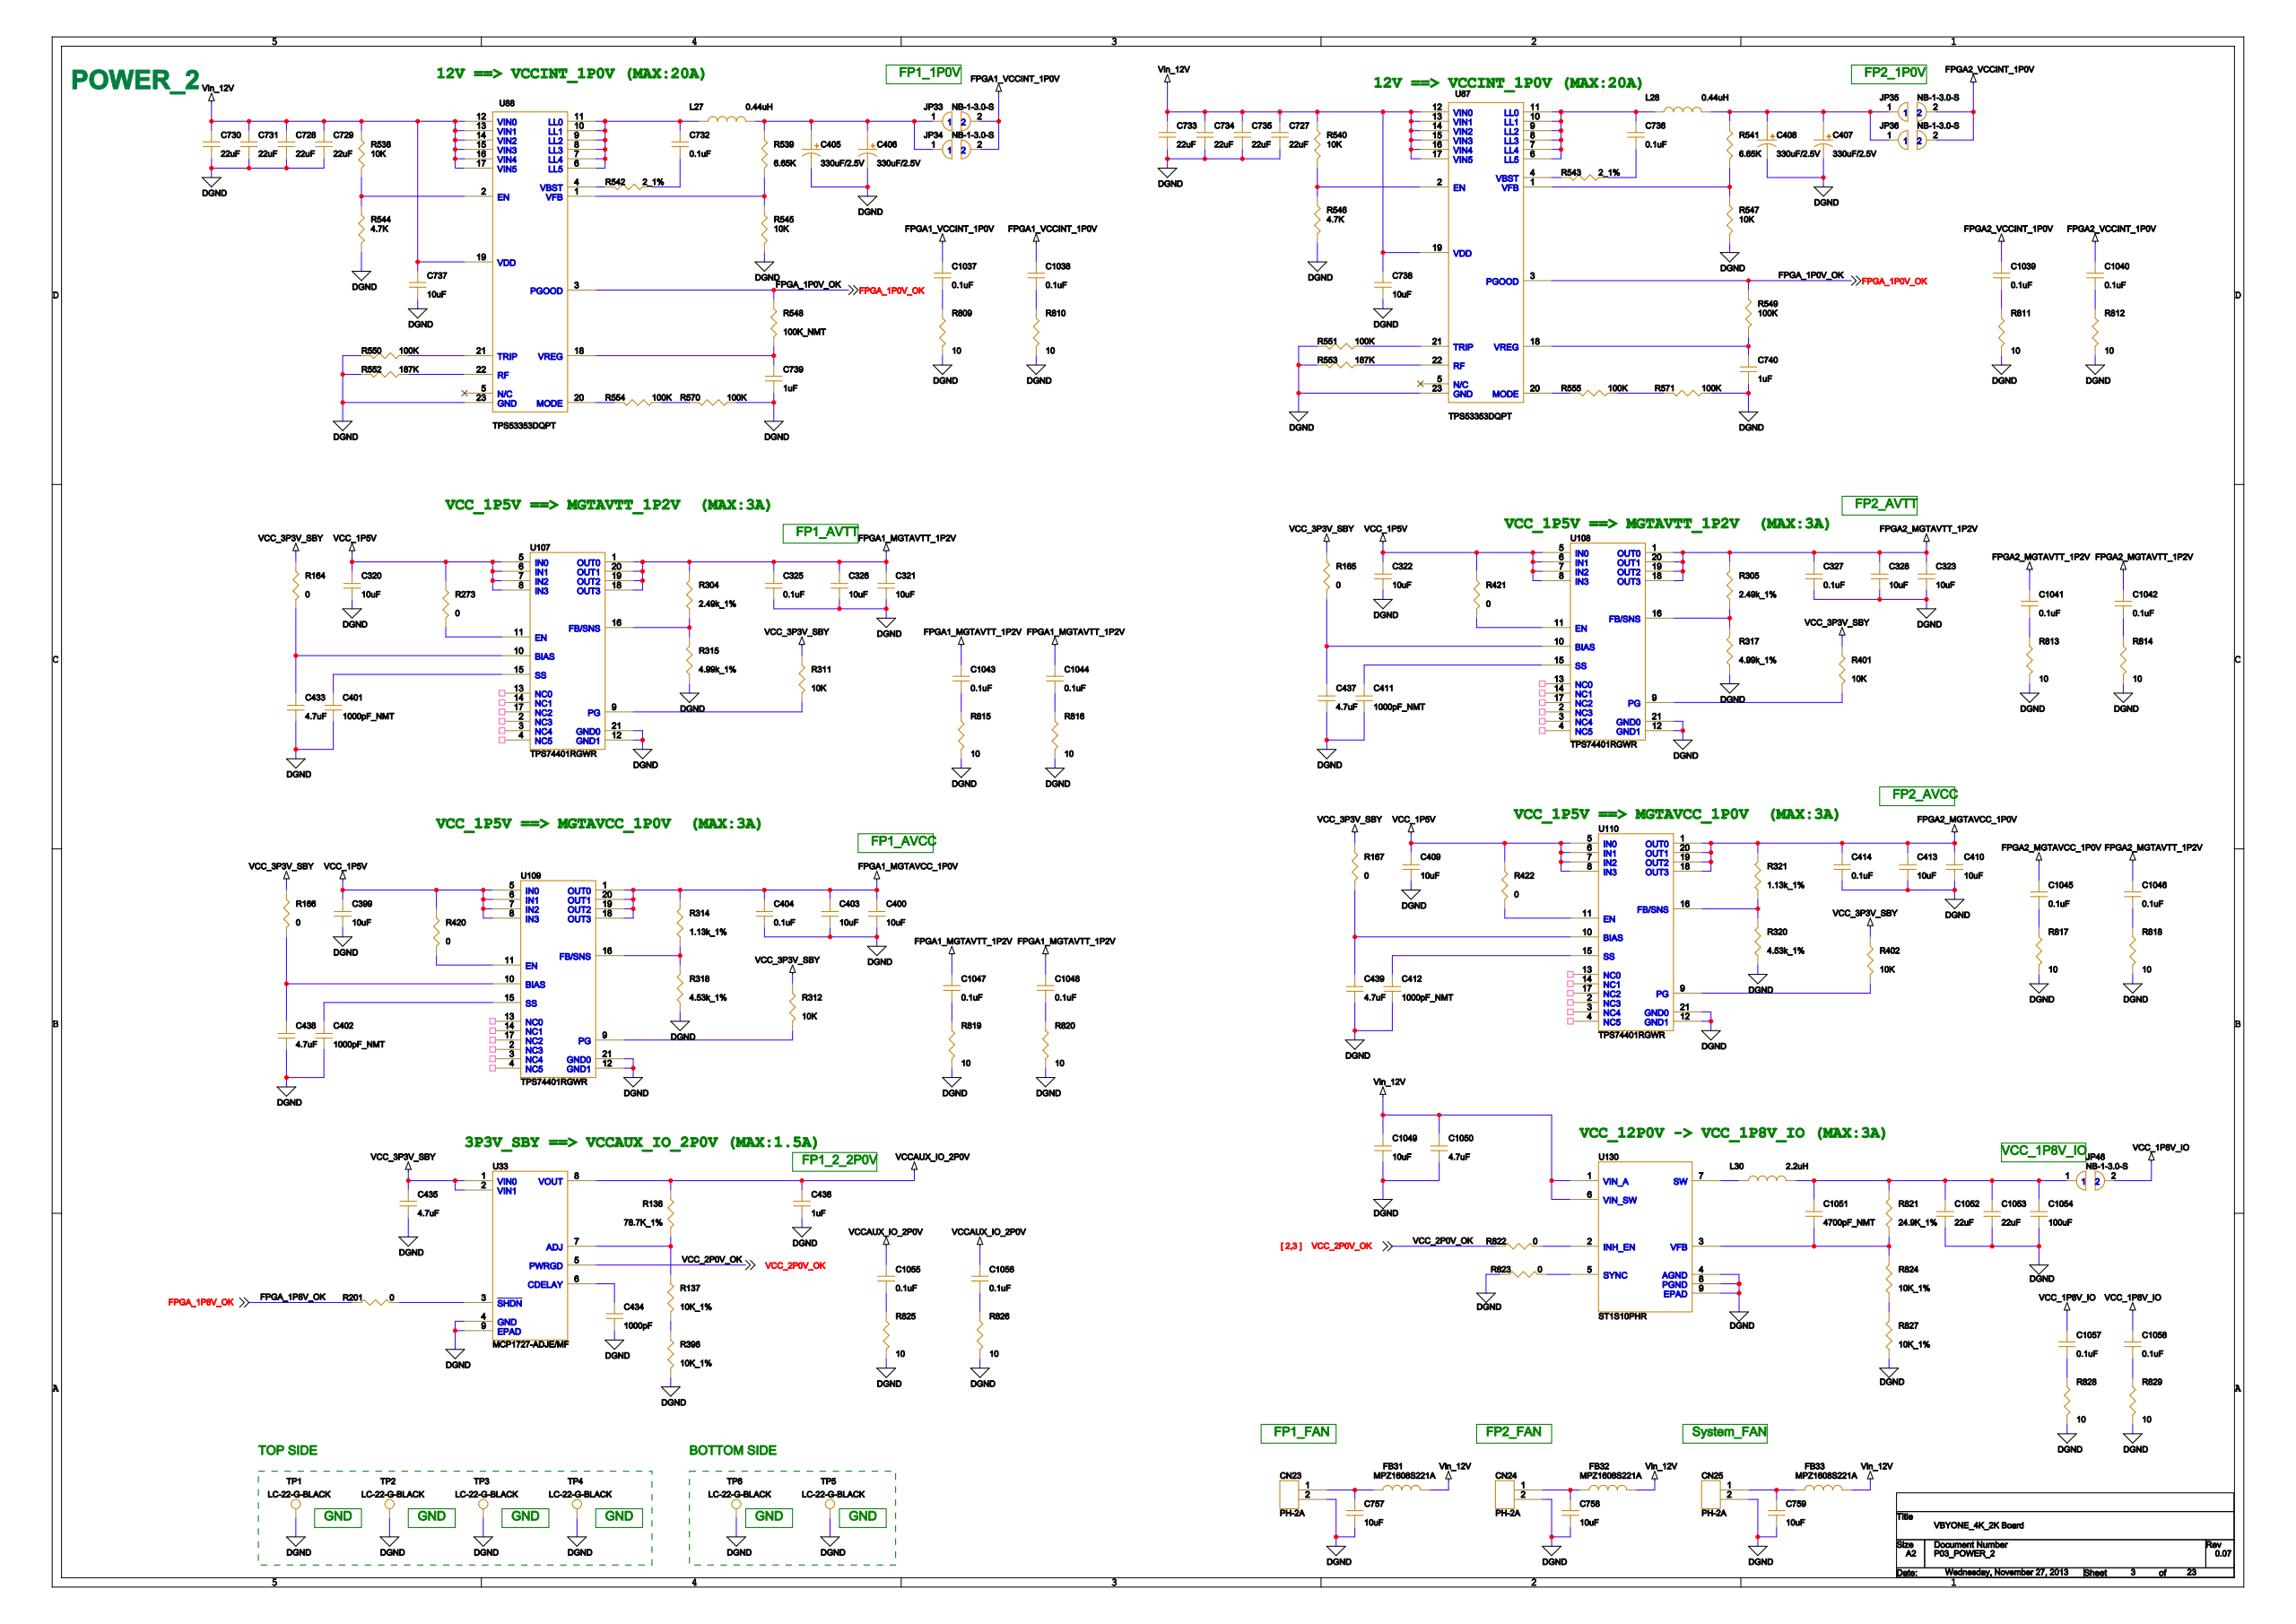Circuit board | Cadence Allegro | 1712 parts | 1495 nets | one sheet of the schematic
Parts on this sheet (reference | value | footprint):
C320 | 10uF | CRC2012RZAS
C321 | 10uF | CRC2012RZAS
C322 | 10uF | CRC2012RZAS
C323 | 10uF | CRC2012RZAS
C325 | 0.1uF | CRC1005RZAS
C326 | 10uF | CRC2012RZAS
C327 | 0.1uF | CRC1005RZAS
C328 | 10uF | CRC2012RZAS
C399 | 10uF | CRC2012RZAS
C400 | 10uF | CRC2012RZAS
C401 | 1000pF_NMT | CRC1608RZAS
C402 | 1000pF_NMT | CRC1608RZAS
C403 | 10uF | CRC2012RZAS
C404 | 0.1uF | CRC1005RZAS
C405 | 330uF/2.5V | CEC3528RZAS
C406 | 330uF/2.5V | CEC3528RZAS
C407 | 330uF/2.5V | CEC3528RZAS
C408 | 330uF/2.5V | CEC3528RZAS
C409 | 10uF | CRC2012RZAS
C410 | 10uF | CRC2012RZAS
C411 | 1000pF_NMT | CRC1608RZAS
C412 | 1000pF_NMT | CRC1608RZAS
C413 | 10uF | CRC2012RZAS
C414 | 0.1uF | CRC1005RZAS
C433 | 4.7uF | CRC1608RZAS
C434 | 1000pF | CRC1608RZAS
C435 | 4.7uF | CRC1608RZAS
C436 | 1uF | CRC1608RZAS
C437 | 4.7uF | CRC1608RZAS
C438 | 4.7uF | CRC1608RZAS
C439 | 4.7uF | CRC1608RZAS
C727 | 22uF | CRC3225RZAS
C728 | 22uF | CRC3225RZAS
C729 | 22uF | CRC3225RZAS
C730 | 22uF | CRC3225RZAS
C731 | 22uF | CRC3225RZAS
C732 | 0.1uF | CRC1005RZAS
C733 | 22uF | CRC3225RZAS
C734 | 22uF | CRC3225RZAS
C735 | 22uF | CRC3225RZAS
C736 | 0.1uF | CRC1005RZAS
C737 | 10uF | CRC2012RZAS
C738 | 10uF | CRC2012RZAS
C739 | 1uF | CRC1608RZAS
C740 | 1uF | CRC1608RZAS
C757 | 10uF | CRC2012RZAS
C758 | 10uF | CRC2012RZAS
C759 | 10uF | CRC2012RZAS
C1037 | 0.1uF | CRC1005RZAS
C1038 | 0.1uF | CRC1005RZAS
C1039 | 0.1uF | CRC1005RZAS
C1040 | 0.1uF | CRC1005RZAS
C1041 | 0.1uF | CRC1005RZAS
C1042 | 0.1uF | CRC1005RZAS
C1043 | 0.1uF | CRC1005RZAS
C1044 | 0.1uF | CRC1005RZAS
C1045 | 0.1uF | CRC1005RZAS
C1046 | 0.1uF | CRC1005RZAS
C1047 | 0.1uF | CRC1005RZAS
C1048 | 0.1uF | CRC1005RZAS
C1049 | 10uF | CRC2012RZAS
C1050 | 4.7uF | CRC1608RZAS
C1051 | 4700pF_NMT | CRC1608RZAS
C1052 | 22uF | CRC3225RZAS
C1053 | 22uF | CRC3225RZAS
C1054 | 100uF | CRC3225RZAS
C1055 | 0.1uF | CRC1005RZAS
C1056 | 0.1uF | CRC1005RZAS
C1057 | 0.1uF | CRC1005RZAS
C1058 | 0.1uF | CRC1005RZAS
CN23 | PH-2A | CND002LJAS
CN24 | PH-2A | CND002LJAS
CN25 | PH-2A | CND002LJAS
FB31 | MPZ1608S221A | LSC1608RZAS
FB32 | MPZ1608S221A | LSC1608RZAS
FB33 | MPZ1608S221A | LSC1608RZAS
JP33 | NB-1-3.0-S | CUTLAND35
JP34 | NB-1-3.0-S | CUTLAND35
JP35 | NB-1-3.0-S | CUTLAND35
JP36 | NB-1-3.0-S | CUTLAND35
JP46 | NB-1-3.0-S | CUTLAND35
L27 | 0.44uH | LSC002RZOS
L28 | 0.44uH | LSC002RZOS
L30 | 2.2uH | LSC5247RZAS
R136 | 78.7K_1% | CRC1608RZAS
R137 | 10K_1% | CRC1005RZAS
R164 | 0 | CRC1608RZAS
R165 | 0 | CRC1608RZAS
R166 | 0 | CRC1608RZAS
R167 | 0 | CRC1608RZAS
R201 | 0 | CRC1608RZAS
R273 | 0 | CRC1608RZAS
R304 | 2.49k_1% | CRC1608RZAS
R305 | 2.49k_1% | CRC1608RZAS
R311 | 10K | CRC1005RZAS
R312 | 10K | CRC1005RZAS
R314 | 1.13k_1% | CRC1608RZAS
R315 | 4.99k_1% | CRC1608RZAS
R317 | 4.99k_1% | CRC1608RZAS
R318 | 4.53k_1% | CRC1608RZAS
R320 | 4.53k_1% | CRC1608RZAS
R321 | 1.13k_1% | CRC1608RZAS
R396 | 10K_1% | CRC1005RZAS
R401 | 10K | CRC1005RZAS
R402 | 10K | CRC1005RZAS
R420 | 0 | CRC1608RZAS
R421 | 0 | CRC1608RZAS
R422 | 0 | CRC1608RZAS
R538 | 10K | CRC1005RZAS
R539 | 6.65K | CRC1608RZAS
R540 | 10K | CRC1005RZAS
R541 | 6.65K | CRC1608RZAS
R542 | 2_1% | CRC1608RZAS
R543 | 2_1% | CRC1608RZAS
R544 | 4.7K | CRC1005RZAS
R545 | 10K | CRC1005RZAS
R546 | 4.7K | CRC1005RZAS
R547 | 10K | CRC1005RZAS
R548 | 100K_NMT | CRC1608RZAS
R549 | 100K | CRC1608RZAS
R550 | 100K | CRC1608RZAS
R551 | 100K | CRC1608RZAS
R552 | 187K | CRC1608RZAS
R553 | 187K | CRC1608RZAS
R554 | 100K | CRC1608RZAS
R555 | 100K | CRC1608RZAS
R570 | 100K | CRC1608RZAS
R571 | 100K | CRC1608RZAS
R809 | 10 | CRC1005RZAS
R810 | 10 | CRC1005RZAS
R811 | 10 | CRC1005RZAS
R812 | 10 | CRC1005RZAS
R813 | 10 | CRC1005RZAS
R814 | 10 | CRC1005RZAS
R815 | 10 | CRC1005RZAS
R816 | 10 | CRC1005RZAS
R817 | 10 | CRC1005RZAS
R818 | 10 | CRC1005RZAS
R819 | 10 | CRC1005RZAS
R820 | 10 | CRC1005RZAS
R821 | 24.9K_1% | CRC1608RZAS
R822 | 0 | CRC1608RZAS
R823 | 0 | CRC1608RZAS
R824 | 10K_1% | CRC1005RZAS
R825 | 10 | CRC1005RZAS
R826 | 10 | CRC1005RZAS
R827 | 10K_1% | CRC1005RZAS
R828 | 10 | CRC1005RZAS
R829 | 10 | CRC1005RZAS
TP1 | LC-22-G-BLACK | TPD001LZBS
TP2 | LC-22-G-BLACK | TPD001LZBS
TP3 | LC-22-G-BLACK | TPD001LZBS
TP4 | LC-22-G-BLACK | TPD001LZBS
TP5 | LC-22-G-BLACK | TPD001LZBS
TP6 | LC-22-G-BLACK | TPD001LZBS
U33 | MCP1727-ADJE/MF | SOC008REDS
U87 | TPS53353DQPT | SOC022RCAS
U88 | TPS53353DQPT | SOC022RCAS
U107 | TPS74401RGWR | QFN020REAS
U108 | TPS74401RGWR | QFN020REAS
U109 | TPS74401RGWR | QFN020REAS
U110 | TPS74401RGWR | QFN020REAS
U130 | ST1S10PHR | SOC008RHFT
Nets of these parts (net: part-pin ...):
DGND: C320-1 C321-1 C322-1 C323-1 C325-1 C326-1 C327-1 C328-1 C399-1 C400-1 C401-1 C402-1 C403-1 C404-1 C405-2 C406-2 C407-2 C408-2 C409-1 C410-1 C411-1 C412-1 C413-1 C414-1 C433-1 C434-2 C435-2 C436-2 C437-1 C438-1 C439-1 C727-2 C728-2 C729-2 C730-2 C731-2 C733-2 C734-2 C735-2 C737-2 C738-2 C739-2 C740-2 C757-2 C758-2 C759-2 C1049-1 C1050-1 C1052-1 C1053-1 C1054-1 CN23-2 CN24-2 CN25-2 R315-1 R317-1 R318-1 R320-1 R396-2 R544-2 R545-2 R546-2 R547-2 R550-2 R551-2 R552-2 R553-2 R570-1 R571-1 R809-2 R810-2 R811-2 R812-2 R813-2 R814-2 R815-2 R816-2 R817-2 R818-2 R819-2 R820-2 R823-1 R825-2 R826-2 R827-1 R828-2 R829-2 TP1-1 TP2-1 TP3-1 TP4-1 TP5-1 TP6-1 U33-4 U33-9 U107-12 U107-21 U108-12 U108-21 U109-12 U109-21 U110-12 U110-21 U130-4 U130-8 U130-9 U87-23 U88-23
VCC_1P5V: C320-2 C322-2 C399-2 C409-2 R273-1 R420-1 R421-1 R422-1 U107-5 U107-6 U107-7 U107-8 U108-5 U108-6 U108-7 U108-8 U109-5 U109-6 U109-7 U109-8 U110-5 U110-6 U110-7 U110-8
VCC_3P3V_SBY: C435-1 R164-1 R165-1 R166-1 R167-1 R311-1 R312-1 R401-1 R402-1 U33-1 U33-2
VIN_12V: C727-1 C728-1 C729-1 C730-1 C731-1 C733-1 C734-1 C735-1 C737-1 C738-1 C1049-2 C1050-2 FB31-2 FB32-2 FB33-2 R538-1 R540-1 U130-1 U130-6 U87-12 U87-13 U87-14 U87-15 U87-16 U87-17 U87-19 U88-12 U88-13 U88-14 U88-15 U88-16 U88-17 U88-19
FPGA1_VCCINT_1P0V: C1037-1 C1038-1 JP33-2 JP34-2
N19956360: C1037-2 R809-1
N19956388: C1038-2 R810-1
FPGA2_VCCINT_1P0V: C1039-1 C1040-1 JP35-2 JP36-2
N19958375: C1039-2 R811-1
N19958403: C1040-2 R812-1
FPGA2_MGTAVTT_1P2V: C323-2 C327-2 C328-2 C1041-1 C1042-1 C1046-1 R305-2 U108-1 U108-18 U108-19 U108-20
N19958657: C1041-2 R813-1
N19958686: C1042-2 R814-1
FPGA1_MGTAVTT_1P2V: C321-2 C325-2 C326-2 C1043-1 C1044-1 C1047-1 C1048-1 R304-2 U107-1 U107-18 U107-19 U107-20
N19956853: C1043-2 R815-1
N19956885: C1044-2 R816-1
FPGA2_MGTAVCC_1P0V: C410-2 C413-2 C414-2 C1045-1 R321-2 U110-1 U110-18 U110-19 U110-20
N19958984: C1045-2 R817-1
N19958997: C1046-2 R818-1
N19957348: C1047-2 R819-1
N19957380: C1048-2 R820-1
VCCAUX_IO_2P0V: C436-1 C1055-1 C1056-1 R136-1 U33-8
N19957622: C1055-2 R825-1
N19957654: C1056-2 R826-1
VCC_1P8V_IO: C1057-1 C1058-1 JP46-2
N19959361: C1057-2 R828-1
N19959378: C1058-2 R829-1
FPGA1_MGTAVCC_1P0V: C400-2 C403-2 C404-2 R314-2 U109-1 U109-18 U109-19 U109-20
N18061222: C757-1 CN23-1 FB31-1
N18061424: C758-1 CN24-1 FB32-1
N18061628: C759-1 CN25-1 FB33-1
N17840635: C433-2 R164-2 U107-10
N17858006: C437-2 R165-2 U108-10
N17904658: C438-2 R166-2 U109-10
N17904876: C439-2 R167-2 U110-10
N19937143: C1051-1 R821-1 R824-2 U130-3
N19937165: C1051-2 C1052-2 C1053-2 C1054-2 JP46-1 L30-2 R821-2
N17799968: C434-1 U33-6
N17159327: C732-1 L27-1 U88-6 U88-7 U88-8 U88-9 U88-10 U88-11
N17159363: C732-2 R542-1
N17160334: C736-1 L28-1 U87-6 U87-7 U87-8 U87-9 U87-10 U87-11
N17160370: C736-2 R543-1
N17159420: C739-1 R548-2 U88-18
N17160427: C740-1 R549-2 U87-18
N17842105: C401-2 U107-15
N17887682: C402-2 U109-15
N17858033: C411-2 U108-15
N17888370: C412-2 U110-15
N17159278: C405-1 C406-1 JP33-1 JP34-1 L27-2 R539-1
N17160285: C407-1 C408-1 JP35-1 JP36-1 L28-2 R541-1
N19937135: L30-1 U130-7
FPGA_1P8V_OK: R201-1
N17813207: R201-2 U33-3
N18322098: R273-2 U107-11
N17904200: R420-2 U109-11
N18322149: R421-2 U108-11
N17904585: R422-2 U110-11
VCC_2P0V_OK: R822-1 U33-5
FPGA_1P0V_OK: R548-1 R549-1 U87-3 U88-3
N19937379: R822-2 U130-2
N19937141: R823-2 U130-5
N17159227: R538-2 R544-1 U88-2
N17160234: R540-2 R546-1 U87-2
N18321913: R311-2 U107-9
N18321969: R312-2 U109-9
N18322020: R401-2 U108-9
N18322072: R402-2 U110-9
N17159404: R539-2 R545-1 U88-1
N17160411: R541-2 R547-1 U87-1
N17772665: R136-2 R137-1 U33-7
N18243360: R137-2 R396-1
N19937302: R824-1 R827-2
N17856330: R304-1 R315-2 U107-16
N17858114: R305-1 R317-2 U108-16
N17887763: R314-1 R318-2 U109-16
N17888451: R320-2 R321-1 U110-16
N17159495: R550-1 U88-21
N17160502: R551-1 U87-21
N18240956: R554-1 R570-2
N17159416: R554-2 U88-20
N18241914: R555-1 R571-2
N17160423: R555-2 U87-20
N17159367: R542-2 U88-4
N17160374: R543-2 U87-4
N17159487: R552-1 U88-22
N17160494: R553-1 U87-22